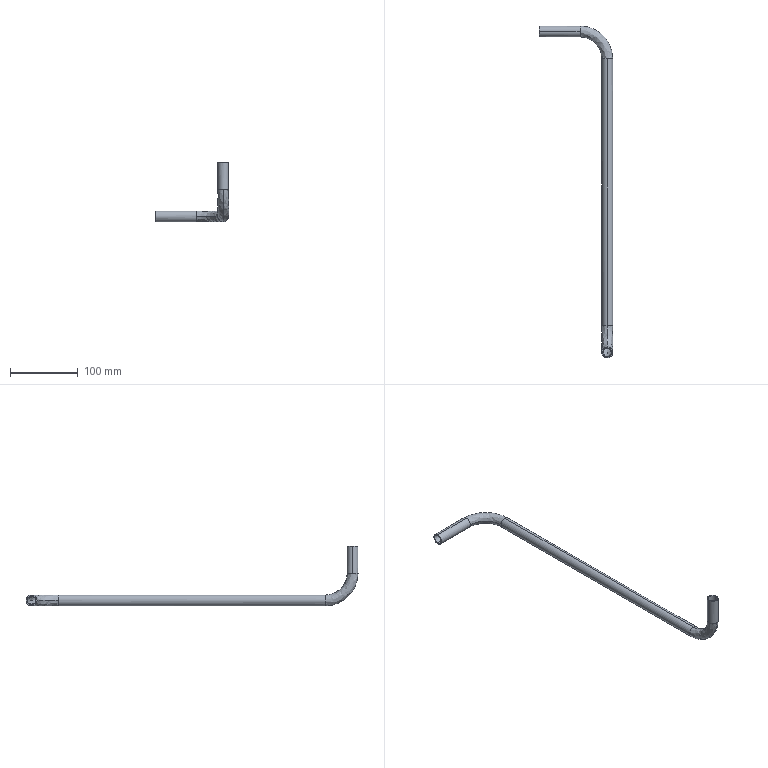Part | STEP file | copper tube 23_default_machined_ | 1 solid | 22 faces | box 108 x 489 x 88 mm | volume 42273 mm3 | cylinder 12 | spline 8 | plane 2 | commonest cylinder face diameters 13 x6 16 x6